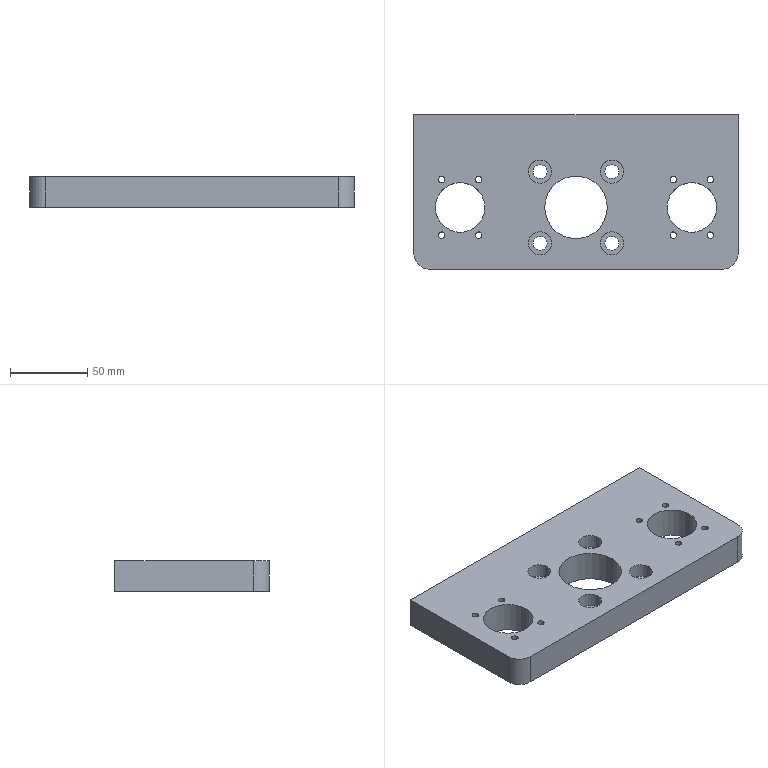Part | STEP file | KF-2212-050-002 | 1 solid | 62 faces | box 210 x 100 x 20 mm | volume 347402 mm3 | cylinder 46 | plane 10 | cone 6 | commonest cylinder face diameters 4.2 x16 9 x8 15 x8 6.8 x6 32.1 x4 20 x2